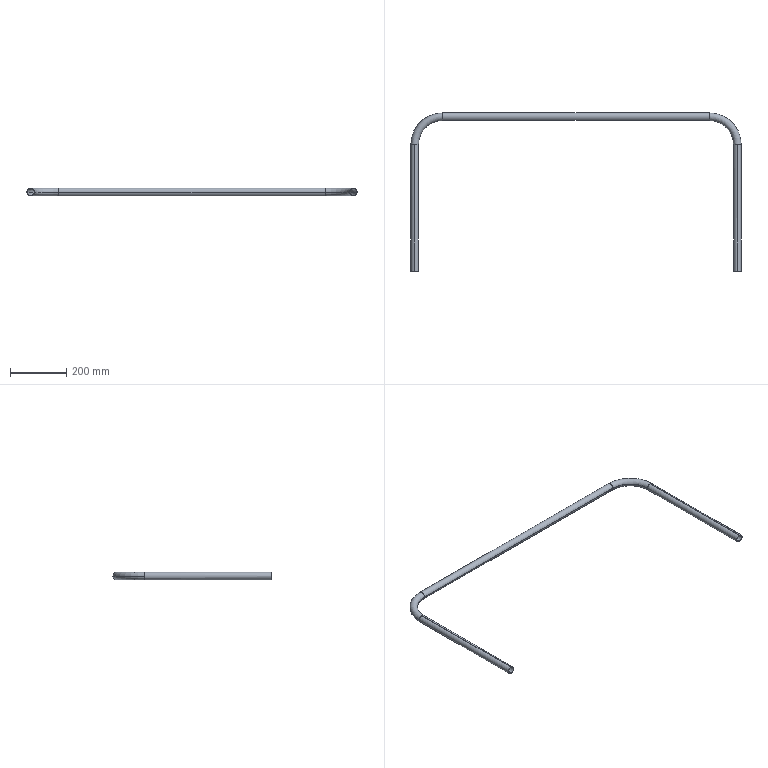Part | SolidWorks | features Sweep 1 | 1 solid | 22 faces | box 1177 x 563.5 x 27 mm | volume 176772 mm3 | cylinder 12 | torus 8 | plane 2 | commonest cylinder face diameters 25 x6 27 x6
STEP:
#1=CARTESIAN_POINT('',(-475.,562.5,0.));
#2=VERTEX_POINT('',#1);
#3=CARTESIAN_POINT('',(-475.,537.5,0.));
#4=VERTEX_POINT('',#3);
#5=CARTESIAN_POINT('',(-475.,550.,0.));
#6=DIRECTION('',(-1.,0.,0.));
#7=DIRECTION('',(0.,1.,0.));
#8=AXIS2_PLACEMENT_3D('',#5,#6,#7);
#9=CIRCLE('',#8,12.5);
#10=EDGE_CURVE('',#2,#4,#9,.T.);
#11=ORIENTED_EDGE('',*,*,#10,.F.);
#12=CARTESIAN_POINT('',(-587.5,450.,0.));
#13=VERTEX_POINT('',#12);
#14=CARTESIAN_POINT('',(-475.,450.,0.));
#15=DIRECTION('',(0.,0.,1.));
#16=DIRECTION('',(1.,0.,0.));
#17=AXIS2_PLACEMENT_3D('',#14,#15,#16);
#18=CIRCLE('',#17,112.5);
#19=EDGE_CURVE('',#2,#13,#18,.T.);
#20=ORIENTED_EDGE('',*,*,#19,.T.);
#21=CARTESIAN_POINT('',(-575.,450.,-12.5));
#22=VERTEX_POINT('',#21);
#23=CARTESIAN_POINT('',(-575.,450.,0.));
#24=DIRECTION('',(0.,-1.,0.));
#25=DIRECTION('',(0.,0.,-1.));
#26=AXIS2_PLACEMENT_3D('',#23,#24,#25);
#27=CIRCLE('',#26,12.5);
#28=EDGE_CURVE('',#13,#22,#27,.T.);
#29=ORIENTED_EDGE('',*,*,#28,.T.);
#30=CARTESIAN_POINT('',(-562.5,450.,0.));
#31=VERTEX_POINT('',#30);
#32=CARTESIAN_POINT('',(-575.,450.,0.));
#33=DIRECTION('',(0.,-1.,0.));
#34=DIRECTION('',(0.,0.,-1.));
#35=AXIS2_PLACEMENT_3D('',#32,#33,#34);
#36=CIRCLE('',#35,12.5);
#37=EDGE_CURVE('',#22,#31,#36,.T.);
#38=ORIENTED_EDGE('',*,*,#37,.T.);
#39=CARTESIAN_POINT('',(-475.,450.,0.));
#40=DIRECTION('',(0.,0.,1.));
#41=DIRECTION('',(1.,0.,0.));
#42=AXIS2_PLACEMENT_3D('',#39,#40,#41);
#43=CIRCLE('',#42,87.5);
#44=EDGE_CURVE('',#4,#31,#43,.T.);
#45=ORIENTED_EDGE('',*,*,#44,.F.);
#46=EDGE_LOOP('',(#11,#20,#29,#38,#45));
#47=FACE_OUTER_BOUND('',#46,.T.);
#48=CARTESIAN_POINT('',(-475.,450.,0.));
#49=DIRECTION('',(0.,0.,1.));
#50=DIRECTION('',(1.,0.,0.));
#51=AXIS2_PLACEMENT_3D('',#48,#49,#50);
#52=TOROIDAL_SURFACE('',#51,100.,12.5);
#53=ADVANCED_FACE('',(#47),#52,.F.);
#54=CARTESIAN_POINT('',(587.5,450.,0.));
#55=VERTEX_POINT('',#54);
#56=CARTESIAN_POINT('',(575.,450.,-12.5));
#57=VERTEX_POINT('',#56);
#58=CARTESIAN_POINT('',(575.,450.,0.));
#59=DIRECTION('',(0.,1.,0.));
#60=DIRECTION('',(1.,0.,0.));
#61=AXIS2_PLACEMENT_3D('',#58,#59,#60);
#62=CIRCLE('',#61,12.5);
#63=EDGE_CURVE('',#55,#57,#62,.T.);
#64=ORIENTED_EDGE('',*,*,#63,.F.);
#65=CARTESIAN_POINT('',(475.,562.5,0.));
#66=VERTEX_POINT('',#65);
#67=CARTESIAN_POINT('',(475.,450.,0.));
#68=DIRECTION('',(0.,0.,1.));
#69=DIRECTION('',(1.,0.,0.));
#70=AXIS2_PLACEMENT_3D('',#67,#68,#69);
#71=CIRCLE('',#70,112.5);
#72=EDGE_CURVE('',#55,#66,#71,.T.);
#73=ORIENTED_EDGE('',*,*,#72,.T.);
#74=CARTESIAN_POINT('',(475.,537.5,0.));
#75=VERTEX_POINT('',#74);
#76=CARTESIAN_POINT('',(475.,550.,0.));
#77=DIRECTION('',(-1.,0.,0.));
#78=DIRECTION('',(0.,-1.,0.));
#79=AXIS2_PLACEMENT_3D('',#76,#77,#78);
#80=CIRCLE('',#79,12.5);
#81=EDGE_CURVE('',#66,#75,#80,.T.);
#82=ORIENTED_EDGE('',*,*,#81,.T.);
#83=CARTESIAN_POINT('',(562.5,450.,0.));
#84=VERTEX_POINT('',#83);
#85=CARTESIAN_POINT('',(475.,450.,0.));
#86=DIRECTION('',(0.,0.,1.));
#87=DIRECTION('',(1.,0.,0.));
#88=AXIS2_PLACEMENT_3D('',#85,#86,#87);
#89=CIRCLE('',#88,87.5);
#90=EDGE_CURVE('',#84,#75,#89,.T.);
#91=ORIENTED_EDGE('',*,*,#90,.F.);
#92=CARTESIAN_POINT('',(575.,450.,0.));
#93=DIRECTION('',(0.,1.,0.));
#94=DIRECTION('',(1.,0.,0.));
#95=AXIS2_PLACEMENT_3D('',#92,#93,#94);
#96=CIRCLE('',#95,12.5);
#97=EDGE_CURVE('',#57,#84,#96,.T.);
#98=ORIENTED_EDGE('',*,*,#97,.F.);
#99=EDGE_LOOP('',(#64,#73,#82,#91,#98));
#100=FACE_OUTER_BOUND('',#99,.T.);
#101=CARTESIAN_POINT('',(475.,450.,0.));
#102=DIRECTION('',(0.,0.,1.));
#103=DIRECTION('',(1.,0.,0.));
#104=AXIS2_PLACEMENT_3D('',#101,#102,#103);
#105=TOROIDAL_SURFACE('',#104,100.,12.5);
#106=ADVANCED_FACE('',(#100),#105,.F.);
#107=CARTESIAN_POINT('',(-475.,536.5,0.));
#108=VERTEX_POINT('',#107);
#109=CARTESIAN_POINT('',(-475.,563.5,0.));
#110=VERTEX_POINT('',#109);
#111=CARTESIAN_POINT('',(-475.,550.,0.));
#112=DIRECTION('',(-1.,0.,0.));
#113=DIRECTION('',(0.,0.,1.));
#114=AXIS2_PLACEMENT_3D('',#111,#112,#113);
#115=CIRCLE('',#114,13.5);
#116=EDGE_CURVE('',#108,#110,#115,.T.);
#117=ORIENTED_EDGE('',*,*,#116,.T.);
#118=CARTESIAN_POINT('',(-588.5,450.,0.));
#119=VERTEX_POINT('',#118);
#120=CARTESIAN_POINT('',(-475.,450.,0.));
#121=DIRECTION('',(0.,0.,1.));
#122=DIRECTION('',(1.,0.,0.));
#123=AXIS2_PLACEMENT_3D('',#120,#121,#122);
#124=CIRCLE('',#123,113.5);
#125=EDGE_CURVE('',#110,#119,#124,.T.);
#126=ORIENTED_EDGE('',*,*,#125,.T.);
#127=CARTESIAN_POINT('',(-575.,450.,13.5));
#128=VERTEX_POINT('',#127);
#129=CARTESIAN_POINT('',(-575.,450.,0.));
#130=DIRECTION('',(0.,-1.,0.));
#131=DIRECTION('',(0.,0.,1.));
#132=AXIS2_PLACEMENT_3D('',#129,#130,#131);
#133=CIRCLE('',#132,13.5);
#134=EDGE_CURVE('',#128,#119,#133,.T.);
#135=ORIENTED_EDGE('',*,*,#134,.F.);
#136=CARTESIAN_POINT('',(-561.5,450.,0.));
#137=VERTEX_POINT('',#136);
#138=CARTESIAN_POINT('',(-575.,450.,0.));
#139=DIRECTION('',(0.,-1.,0.));
#140=DIRECTION('',(0.,0.,1.));
#141=AXIS2_PLACEMENT_3D('',#138,#139,#140);
#142=CIRCLE('',#141,13.5);
#143=EDGE_CURVE('',#137,#128,#142,.T.);
#144=ORIENTED_EDGE('',*,*,#143,.F.);
#145=CARTESIAN_POINT('',(-475.,450.,0.));
#146=DIRECTION('',(0.,0.,1.));
#147=DIRECTION('',(1.,0.,0.));
#148=AXIS2_PLACEMENT_3D('',#145,#146,#147);
#149=CIRCLE('',#148,86.5);
#150=EDGE_CURVE('',#108,#137,#149,.T.);
#151=ORIENTED_EDGE('',*,*,#150,.F.);
#152=EDGE_LOOP('',(#117,#126,#135,#144,#151));
#153=FACE_OUTER_BOUND('',#152,.T.);
#154=CARTESIAN_POINT('',(-475.,450.,0.));
#155=DIRECTION('',(0.,0.,1.));
#156=DIRECTION('',(1.,0.,0.));
#157=AXIS2_PLACEMENT_3D('',#154,#155,#156);
#158=TOROIDAL_SURFACE('',#157,100.,13.5);
#159=ADVANCED_FACE('',(#153),#158,.T.);
#160=CARTESIAN_POINT('',(575.,450.,13.5));
#161=VERTEX_POINT('',#160);
#162=CARTESIAN_POINT('',(588.5,450.,0.));
#163=VERTEX_POINT('',#162);
#164=CARTESIAN_POINT('',(575.,450.,0.));
#165=DIRECTION('',(0.,1.,0.));
#166=DIRECTION('',(0.,0.,1.));
#167=AXIS2_PLACEMENT_3D('',#164,#165,#166);
#168=CIRCLE('',#167,13.5);
#169=EDGE_CURVE('',#161,#163,#168,.T.);
#170=ORIENTED_EDGE('',*,*,#169,.T.);
#171=CARTESIAN_POINT('',(475.,563.5,0.));
#172=VERTEX_POINT('',#171);
#173=CARTESIAN_POINT('',(475.,450.,0.));
#174=DIRECTION('',(0.,0.,1.));
#175=DIRECTION('',(1.,0.,0.));
#176=AXIS2_PLACEMENT_3D('',#173,#174,#175);
#177=CIRCLE('',#176,113.5);
#178=EDGE_CURVE('',#163,#172,#177,.T.);
#179=ORIENTED_EDGE('',*,*,#178,.T.);
#180=CARTESIAN_POINT('',(475.,536.5,0.));
#181=VERTEX_POINT('',#180);
#182=CARTESIAN_POINT('',(475.,550.,0.));
#183=DIRECTION('',(-1.,0.,0.));
#184=DIRECTION('',(0.,0.,1.));
#185=AXIS2_PLACEMENT_3D('',#182,#183,#184);
#186=CIRCLE('',#185,13.5);
#187=EDGE_CURVE('',#181,#172,#186,.T.);
#188=ORIENTED_EDGE('',*,*,#187,.F.);
#189=CARTESIAN_POINT('',(561.5,450.,0.));
#190=VERTEX_POINT('',#189);
#191=CARTESIAN_POINT('',(475.,450.,0.));
#192=DIRECTION('',(0.,0.,1.));
#193=DIRECTION('',(1.,0.,0.));
#194=AXIS2_PLACEMENT_3D('',#191,#192,#193);
#195=CIRCLE('',#194,86.5);
#196=EDGE_CURVE('',#190,#181,#195,.T.);
#197=ORIENTED_EDGE('',*,*,#196,.F.);
#198=CARTESIAN_POINT('',(575.,450.,0.));
#199=DIRECTION('',(0.,1.,0.));
#200=DIRECTION('',(0.,0.,1.));
#201=AXIS2_PLACEMENT_3D('',#198,#199,#200);
#202=CIRCLE('',#201,13.5);
#203=EDGE_CURVE('',#190,#161,#202,.T.);
#204=ORIENTED_EDGE('',*,*,#203,.T.);
#205=EDGE_LOOP('',(#170,#179,#188,#197,#204));
#206=FACE_OUTER_BOUND('',#205,.T.);
#207=CARTESIAN_POINT('',(475.,450.,0.));
#208=DIRECTION('',(0.,0.,1.));
#209=DIRECTION('',(1.,0.,0.));
#210=AXIS2_PLACEMENT_3D('',#207,#208,#209);
#211=TOROIDAL_SURFACE('',#210,100.,13.5);
#212=ADVANCED_FACE('',(#206),#211,.T.);
#213=CARTESIAN_POINT('',(-575.,450.,12.5));
#214=VERTEX_POINT('',#213);
#215=CARTESIAN_POINT('',(-575.,450.,0.));
#216=DIRECTION('',(0.,-1.,0.));
#217=DIRECTION('',(0.,0.,-1.));
#218=AXIS2_PLACEMENT_3D('',#215,#216,#217);
#219=CIRCLE('',#218,12.5);
#220=EDGE_CURVE('',#214,#13,#219,.T.);
#221=ORIENTED_EDGE('',*,*,#220,.F.);
#222=CARTESIAN_POINT('',(-575.,0.,12.5));
#223=VERTEX_POINT('',#222);
#224=CARTESIAN_POINT('',(-575.,450.,12.5));
#225=DIRECTION('',(0.,-1.,0.));
#226=VECTOR('',#225,1000.);
#227=LINE('',#224,#226);
#228=EDGE_CURVE('',#214,#223,#227,.T.);
#229=ORIENTED_EDGE('',*,*,#228,.T.);
#230=CARTESIAN_POINT('',(-575.,0.,-12.5));
#231=VERTEX_POINT('',#230);
#232=CARTESIAN_POINT('',(-575.,0.,0.));
#233=DIRECTION('',(0.,-1.,0.));
#234=DIRECTION('',(0.,0.,-1.));
#235=AXIS2_PLACEMENT_3D('',#232,#233,#234);
#236=CIRCLE('',#235,12.5);
#237=EDGE_CURVE('',#223,#231,#236,.T.);
#238=ORIENTED_EDGE('',*,*,#237,.T.);
#239=CARTESIAN_POINT('',(-575.,450.,-12.5));
#240=DIRECTION('',(0.,-1.,0.));
#241=VECTOR('',#240,1000.);
#242=LINE('',#239,#241);
#243=EDGE_CURVE('',#22,#231,#242,.T.);
#244=ORIENTED_EDGE('',*,*,#243,.F.);
#245=ORIENTED_EDGE('',*,*,#28,.F.);
#246=EDGE_LOOP('',(#221,#229,#238,#244,#245));
#247=FACE_OUTER_BOUND('',#246,.T.);
#248=CARTESIAN_POINT('',(-575.,450.,0.));
#249=DIRECTION('',(0.,-1.,0.));
#250=DIRECTION('',(0.,0.,-1.));
#251=AXIS2_PLACEMENT_3D('',#248,#249,#250);
#252=CYLINDRICAL_SURFACE('',#251,12.5);
#253=ADVANCED_FACE('',(#247),#252,.F.);
#254=ORIENTED_EDGE('',*,*,#81,.F.);
#255=CARTESIAN_POINT('',(475.,562.5,0.));
#256=DIRECTION('',(-1.,0.,0.));
#257=VECTOR('',#256,1000.);
#258=LINE('',#255,#257);
#259=EDGE_CURVE('',#66,#2,#258,.T.);
#260=ORIENTED_EDGE('',*,*,#259,.T.);
#261=ORIENTED_EDGE('',*,*,#10,.T.);
#262=CARTESIAN_POINT('',(475.,537.5,0.));
#263=DIRECTION('',(-1.,0.,0.));
#264=VECTOR('',#263,1000.);
#265=LINE('',#262,#264);
#266=EDGE_CURVE('',#75,#4,#265,.T.);
#267=ORIENTED_EDGE('',*,*,#266,.F.);
#268=EDGE_LOOP('',(#254,#260,#261,#267));
#269=FACE_OUTER_BOUND('',#268,.T.);
#270=CARTESIAN_POINT('',(475.,550.,0.));
#271=DIRECTION('',(-1.,0.,0.));
#272=DIRECTION('',(0.,-1.,0.));
#273=AXIS2_PLACEMENT_3D('',#270,#271,#272);
#274=CYLINDRICAL_SURFACE('',#273,12.5);
#275=ADVANCED_FACE('',(#269),#274,.F.);
#276=CARTESIAN_POINT('',(575.,0.,-12.5));
#277=VERTEX_POINT('',#276);
#278=CARTESIAN_POINT('',(575.,0.,12.5));
#279=VERTEX_POINT('',#278);
#280=CARTESIAN_POINT('',(575.,0.,0.));
#281=DIRECTION('',(0.,1.,0.));
#282=DIRECTION('',(0.,0.,1.));
#283=AXIS2_PLACEMENT_3D('',#280,#281,#282);
#284=CIRCLE('',#283,12.5);
#285=EDGE_CURVE('',#277,#279,#284,.T.);
#286=ORIENTED_EDGE('',*,*,#285,.F.);
#287=CARTESIAN_POINT('',(575.,0.,-12.5));
#288=DIRECTION('',(0.,1.,0.));
#289=VECTOR('',#288,1000.);
#290=LINE('',#287,#289);
#291=EDGE_CURVE('',#277,#57,#290,.T.);
#292=ORIENTED_EDGE('',*,*,#291,.T.);
#293=ORIENTED_EDGE('',*,*,#97,.T.);
#294=CARTESIAN_POINT('',(575.,450.,12.5));
#295=VERTEX_POINT('',#294);
#296=CARTESIAN_POINT('',(575.,450.,0.));
#297=DIRECTION('',(0.,1.,0.));
#298=DIRECTION('',(1.,0.,0.));
#299=AXIS2_PLACEMENT_3D('',#296,#297,#298);
#300=CIRCLE('',#299,12.5);
#301=EDGE_CURVE('',#84,#295,#300,.T.);
#302=ORIENTED_EDGE('',*,*,#301,.T.);
#303=CARTESIAN_POINT('',(575.,0.,12.5));
#304=DIRECTION('',(0.,1.,0.));
#305=VECTOR('',#304,1000.);
#306=LINE('',#303,#305);
#307=EDGE_CURVE('',#279,#295,#306,.T.);
#308=ORIENTED_EDGE('',*,*,#307,.F.);
#309=EDGE_LOOP('',(#286,#292,#293,#302,#308));
#310=FACE_OUTER_BOUND('',#309,.T.);
#311=CARTESIAN_POINT('',(575.,0.,0.));
#312=DIRECTION('',(0.,1.,0.));
#313=DIRECTION('',(0.,0.,1.));
#314=AXIS2_PLACEMENT_3D('',#311,#312,#313);
#315=CYLINDRICAL_SURFACE('',#314,12.5);
#316=ADVANCED_FACE('',(#310),#315,.F.);
#317=CARTESIAN_POINT('',(-575.,450.,-13.5));
#318=VERTEX_POINT('',#317);
#319=CARTESIAN_POINT('',(-575.,450.,0.));
#320=DIRECTION('',(0.,-1.,0.));
#321=DIRECTION('',(0.,0.,1.));
#322=AXIS2_PLACEMENT_3D('',#319,#320,#321);
#323=CIRCLE('',#322,13.5);
#324=EDGE_CURVE('',#318,#137,#323,.T.);
#325=ORIENTED_EDGE('',*,*,#324,.T.);
#326=ORIENTED_EDGE('',*,*,#143,.T.);
#327=CARTESIAN_POINT('',(-575.,0.,13.5));
#328=VERTEX_POINT('',#327);
#329=CARTESIAN_POINT('',(-575.,450.,13.5));
#330=DIRECTION('',(0.,-1.,0.));
#331=VECTOR('',#330,1000.);
#332=LINE('',#329,#331);
#333=EDGE_CURVE('',#128,#328,#332,.T.);
#334=ORIENTED_EDGE('',*,*,#333,.T.);
#335=CARTESIAN_POINT('',(-575.,0.,-13.5));
#336=VERTEX_POINT('',#335);
#337=CARTESIAN_POINT('',(-575.,0.,0.));
#338=DIRECTION('',(0.,-1.,0.));
#339=DIRECTION('',(0.,0.,1.));
#340=AXIS2_PLACEMENT_3D('',#337,#338,#339);
#341=CIRCLE('',#340,13.5);
#342=EDGE_CURVE('',#336,#328,#341,.T.);
#343=ORIENTED_EDGE('',*,*,#342,.F.);
#344=CARTESIAN_POINT('',(-575.,450.,-13.5));
#345=DIRECTION('',(0.,-1.,0.));
#346=VECTOR('',#345,1000.);
#347=LINE('',#344,#346);
#348=EDGE_CURVE('',#318,#336,#347,.T.);
#349=ORIENTED_EDGE('',*,*,#348,.F.);
#350=EDGE_LOOP('',(#325,#326,#334,#343,#349));
#351=FACE_OUTER_BOUND('',#350,.T.);
#352=CARTESIAN_POINT('',(-575.,450.,0.));
#353=DIRECTION('',(0.,-1.,0.));
#354=DIRECTION('',(0.,0.,-1.));
#355=AXIS2_PLACEMENT_3D('',#352,#353,#354);
#356=CYLINDRICAL_SURFACE('',#355,13.5);
#357=ADVANCED_FACE('',(#351),#356,.T.);
#358=ORIENTED_EDGE('',*,*,#187,.T.);
#359=CARTESIAN_POINT('',(475.,563.5,0.));
#360=DIRECTION('',(-1.,0.,0.));
#361=VECTOR('',#360,1000.);
#362=LINE('',#359,#361);
#363=EDGE_CURVE('',#172,#110,#362,.T.);
#364=ORIENTED_EDGE('',*,*,#363,.T.);
#365=ORIENTED_EDGE('',*,*,#116,.F.);
#366=CARTESIAN_POINT('',(475.,536.5,0.));
#367=DIRECTION('',(-1.,0.,0.));
#368=VECTOR('',#367,1000.);
#369=LINE('',#366,#368);
#370=EDGE_CURVE('',#181,#108,#369,.T.);
#371=ORIENTED_EDGE('',*,*,#370,.F.);
#372=EDGE_LOOP('',(#358,#364,#365,#371));
#373=FACE_OUTER_BOUND('',#372,.T.);
#374=CARTESIAN_POINT('',(475.,550.,0.));
#375=DIRECTION('',(-1.,0.,0.));
#376=DIRECTION('',(0.,-1.,0.));
#377=AXIS2_PLACEMENT_3D('',#374,#375,#376);
#378=CYLINDRICAL_SURFACE('',#377,13.5);
#379=ADVANCED_FACE('',(#373),#378,.T.);
#380=CARTESIAN_POINT('',(575.,0.,13.5));
#381=VERTEX_POINT('',#380);
#382=CARTESIAN_POINT('',(575.,0.,-13.5));
#383=VERTEX_POINT('',#382);
#384=CARTESIAN_POINT('',(575.,0.,0.));
#385=DIRECTION('',(0.,1.,0.));
#386=DIRECTION('',(0.,0.,1.));
#387=AXIS2_PLACEMENT_3D('',#384,#385,#386);
#388=CIRCLE('',#387,13.5);
#389=EDGE_CURVE('',#381,#383,#388,.T.);
#390=ORIENTED_EDGE('',*,*,#389,.T.);
#391=CARTESIAN_POINT('',(575.,450.,-13.5));
#392=VERTEX_POINT('',#391);
#393=CARTESIAN_POINT('',(575.,0.,-13.5));
#394=DIRECTION('',(0.,1.,0.));
#395=VECTOR('',#394,1000.);
#396=LINE('',#393,#395);
#397=EDGE_CURVE('',#383,#392,#396,.T.);
#398=ORIENTED_EDGE('',*,*,#397,.T.);
#399=CARTESIAN_POINT('',(575.,450.,0.));
#400=DIRECTION('',(0.,1.,0.));
#401=DIRECTION('',(0.,0.,1.));
#402=AXIS2_PLACEMENT_3D('',#399,#400,#401);
#403=CIRCLE('',#402,13.5);
#404=EDGE_CURVE('',#163,#392,#403,.T.);
#405=ORIENTED_EDGE('',*,*,#404,.F.);
#406=ORIENTED_EDGE('',*,*,#169,.F.);
#407=CARTESIAN_POINT('',(575.,0.,13.5));
#408=DIRECTION('',(0.,1.,0.));
#409=VECTOR('',#408,1000.);
#410=LINE('',#407,#409);
#411=EDGE_CURVE('',#381,#161,#410,.T.);
#412=ORIENTED_EDGE('',*,*,#411,.F.);
#413=EDGE_LOOP('',(#390,#398,#405,#406,#412));
#414=FACE_OUTER_BOUND('',#413,.T.);
#415=CARTESIAN_POINT('',(575.,0.,0.));
#416=DIRECTION('',(0.,1.,0.));
#417=DIRECTION('',(0.,0.,1.));
#418=AXIS2_PLACEMENT_3D('',#415,#416,#417);
#419=CYLINDRICAL_SURFACE('',#418,13.5);
#420=ADVANCED_FACE('',(#414),#419,.T.);
#421=ORIENTED_EDGE('',*,*,#333,.F.);
#422=ORIENTED_EDGE('',*,*,#134,.T.);
#423=CARTESIAN_POINT('',(-575.,450.,0.));
#424=DIRECTION('',(0.,-1.,0.));
#425=DIRECTION('',(0.,0.,1.));
#426=AXIS2_PLACEMENT_3D('',#423,#424,#425);
#427=CIRCLE('',#426,13.5);
#428=EDGE_CURVE('',#119,#318,#427,.T.);
#429=ORIENTED_EDGE('',*,*,#428,.T.);
#430=ORIENTED_EDGE('',*,*,#348,.T.);
#431=CARTESIAN_POINT('',(-575.,0.,0.));
#432=DIRECTION('',(0.,-1.,0.));
#433=DIRECTION('',(0.,0.,1.));
#434=AXIS2_PLACEMENT_3D('',#431,#432,#433);
#435=CIRCLE('',#434,13.5);
#436=EDGE_CURVE('',#328,#336,#435,.T.);
#437=ORIENTED_EDGE('',*,*,#436,.F.);
#438=EDGE_LOOP('',(#421,#422,#429,#430,#437));
#439=FACE_OUTER_BOUND('',#438,.T.);
#440=CARTESIAN_POINT('',(-575.,450.,0.));
#441=DIRECTION('',(0.,-1.,0.));
#442=DIRECTION('',(0.,0.,-1.));
#443=AXIS2_PLACEMENT_3D('',#440,#441,#442);
#444=CYLINDRICAL_SURFACE('',#443,13.5);
#445=ADVANCED_FACE('',(#439),#444,.T.);
#446=ORIENTED_EDGE('',*,*,#125,.F.);
#447=CARTESIAN_POINT('',(-475.,550.,0.));
#448=DIRECTION('',(-1.,0.,0.));
#449=DIRECTION('',(0.,0.,1.));
#450=AXIS2_PLACEMENT_3D('',#447,#448,#449);
#451=CIRCLE('',#450,13.5);
#452=EDGE_CURVE('',#110,#108,#451,.T.);
#453=ORIENTED_EDGE('',*,*,#452,.T.);
#454=ORIENTED_EDGE('',*,*,#150,.T.);
#455=ORIENTED_EDGE('',*,*,#324,.F.);
#456=ORIENTED_EDGE('',*,*,#428,.F.);
#457=EDGE_LOOP('',(#446,#453,#454,#455,#456));
#458=FACE_OUTER_BOUND('',#457,.T.);
#459=CARTESIAN_POINT('',(-475.,450.,0.));
#460=DIRECTION('',(0.,0.,1.));
#461=DIRECTION('',(1.,0.,0.));
#462=AXIS2_PLACEMENT_3D('',#459,#460,#461);
#463=TOROIDAL_SURFACE('',#462,100.,13.5);
#464=ADVANCED_FACE('',(#458),#463,.T.);
#465=ORIENTED_EDGE('',*,*,#363,.F.);
#466=CARTESIAN_POINT('',(475.,550.,0.));
#467=DIRECTION('',(-1.,0.,0.));
#468=DIRECTION('',(0.,0.,1.));
#469=AXIS2_PLACEMENT_3D('',#466,#467,#468);
#470=CIRCLE('',#469,13.5);
#471=EDGE_CURVE('',#172,#181,#470,.T.);
#472=ORIENTED_EDGE('',*,*,#471,.T.);
#473=ORIENTED_EDGE('',*,*,#370,.T.);
#474=ORIENTED_EDGE('',*,*,#452,.F.);
#475=EDGE_LOOP('',(#465,#472,#473,#474));
#476=FACE_OUTER_BOUND('',#475,.T.);
#477=CARTESIAN_POINT('',(475.,550.,0.));
#478=DIRECTION('',(-1.,0.,0.));
#479=DIRECTION('',(0.,-1.,0.));
#480=AXIS2_PLACEMENT_3D('',#477,#478,#479);
#481=CYLINDRICAL_SURFACE('',#480,13.5);
#482=ADVANCED_FACE('',(#476),#481,.T.);
#483=ORIENTED_EDGE('',*,*,#178,.F.);
#484=ORIENTED_EDGE('',*,*,#404,.T.);
#485=CARTESIAN_POINT('',(575.,450.,0.));
#486=DIRECTION('',(0.,1.,0.));
#487=DIRECTION('',(0.,0.,1.));
#488=AXIS2_PLACEMENT_3D('',#485,#486,#487);
#489=CIRCLE('',#488,13.5);
#490=EDGE_CURVE('',#392,#190,#489,.T.);
#491=ORIENTED_EDGE('',*,*,#490,.T.);
#492=ORIENTED_EDGE('',*,*,#196,.T.);
#493=ORIENTED_EDGE('',*,*,#471,.F.);
#494=EDGE_LOOP('',(#483,#484,#491,#492,#493));
#495=FACE_OUTER_BOUND('',#494,.T.);
#496=CARTESIAN_POINT('',(475.,450.,0.));
#497=DIRECTION('',(0.,0.,1.));
#498=DIRECTION('',(1.,0.,0.));
#499=AXIS2_PLACEMENT_3D('',#496,#497,#498);
#500=TOROIDAL_SURFACE('',#499,100.,13.5);
#501=ADVANCED_FACE('',(#495),#500,.T.);
#502=ORIENTED_EDGE('',*,*,#397,.F.);
#503=CARTESIAN_POINT('',(575.,0.,0.));
#504=DIRECTION('',(0.,1.,0.));
#505=DIRECTION('',(0.,0.,1.));
#506=AXIS2_PLACEMENT_3D('',#503,#504,#505);
#507=CIRCLE('',#506,13.5);
#508=EDGE_CURVE('',#383,#381,#507,.T.);
#509=ORIENTED_EDGE('',*,*,#508,.T.);
#510=ORIENTED_EDGE('',*,*,#411,.T.);
#511=ORIENTED_EDGE('',*,*,#203,.F.);
#512=ORIENTED_EDGE('',*,*,#490,.F.);
#513=EDGE_LOOP('',(#502,#509,#510,#511,#512));
#514=FACE_OUTER_BOUND('',#513,.T.);
#515=CARTESIAN_POINT('',(575.,0.,0.));
#516=DIRECTION('',(0.,1.,0.));
#517=DIRECTION('',(0.,0.,1.));
#518=AXIS2_PLACEMENT_3D('',#515,#516,#517);
#519=CYLINDRICAL_SURFACE('',#518,13.5);
#520=ADVANCED_FACE('',(#514),#519,.T.);
#521=CARTESIAN_POINT('',(-575.,0.,0.));
#522=DIRECTION('',(0.,-1.,0.));
#523=DIRECTION('',(0.,0.,-1.));
#524=AXIS2_PLACEMENT_3D('',#521,#522,#523);
#525=CIRCLE('',#524,12.5);
#526=EDGE_CURVE('',#231,#223,#525,.T.);
#527=ORIENTED_EDGE('',*,*,#526,.F.);
#528=ORIENTED_EDGE('',*,*,#237,.F.);
#529=EDGE_LOOP('',(#527,#528));
#530=FACE_BOUND('',#529,.T.);
#531=ORIENTED_EDGE('',*,*,#342,.T.);
#532=ORIENTED_EDGE('',*,*,#436,.T.);
#533=EDGE_LOOP('',(#531,#532));
#534=FACE_OUTER_BOUND('',#533,.T.);
#535=CARTESIAN_POINT('',(-575.,0.,0.));
#536=DIRECTION('',(0.,-1.,0.));
#537=DIRECTION('',(0.,0.,1.));
#538=AXIS2_PLACEMENT_3D('',#535,#536,#537);
#539=PLANE('',#538);
#540=ADVANCED_FACE('',(#530,#534),#539,.T.);
#541=CARTESIAN_POINT('',(575.,0.,0.));
#542=DIRECTION('',(0.,1.,0.));
#543=DIRECTION('',(0.,0.,1.));
#544=AXIS2_PLACEMENT_3D('',#541,#542,#543);
#545=CIRCLE('',#544,12.5);
#546=EDGE_CURVE('',#279,#277,#545,.T.);
#547=ORIENTED_EDGE('',*,*,#546,.T.);
#548=ORIENTED_EDGE('',*,*,#285,.T.);
#549=EDGE_LOOP('',(#547,#548));
#550=FACE_BOUND('',#549,.T.);
#551=ORIENTED_EDGE('',*,*,#389,.F.);
#552=ORIENTED_EDGE('',*,*,#508,.F.);
#553=EDGE_LOOP('',(#551,#552));
#554=FACE_OUTER_BOUND('',#553,.T.);
#555=CARTESIAN_POINT('',(575.,0.,0.));
#556=DIRECTION('',(0.,1.,0.));
#557=DIRECTION('',(0.,0.,1.));
#558=AXIS2_PLACEMENT_3D('',#555,#556,#557);
#559=PLANE('',#558);
#560=ADVANCED_FACE('',(#550,#554),#559,.F.);
#561=ORIENTED_EDGE('',*,*,#228,.F.);
#562=CARTESIAN_POINT('',(-575.,450.,0.));
#563=DIRECTION('',(0.,-1.,0.));
#564=DIRECTION('',(0.,0.,-1.));
#565=AXIS2_PLACEMENT_3D('',#562,#563,#564);
#566=CIRCLE('',#565,12.5);
#567=EDGE_CURVE('',#31,#214,#566,.T.);
#568=ORIENTED_EDGE('',*,*,#567,.F.);
#569=ORIENTED_EDGE('',*,*,#37,.F.);
#570=ORIENTED_EDGE('',*,*,#243,.T.);
#571=ORIENTED_EDGE('',*,*,#526,.T.);
#572=EDGE_LOOP('',(#561,#568,#569,#570,#571));
#573=FACE_OUTER_BOUND('',#572,.T.);
#574=CARTESIAN_POINT('',(-575.,450.,0.));
#575=DIRECTION('',(0.,-1.,0.));
#576=DIRECTION('',(0.,0.,-1.));
#577=AXIS2_PLACEMENT_3D('',#574,#575,#576);
#578=CYLINDRICAL_SURFACE('',#577,12.5);
#579=ADVANCED_FACE('',(#573),#578,.F.);
#580=ORIENTED_EDGE('',*,*,#19,.F.);
#581=CARTESIAN_POINT('',(-475.,550.,0.));
#582=DIRECTION('',(-1.,0.,0.));
#583=DIRECTION('',(0.,1.,0.));
#584=AXIS2_PLACEMENT_3D('',#581,#582,#583);
#585=CIRCLE('',#584,12.5);
#586=EDGE_CURVE('',#4,#2,#585,.T.);
#587=ORIENTED_EDGE('',*,*,#586,.F.);
#588=ORIENTED_EDGE('',*,*,#44,.T.);
#589=ORIENTED_EDGE('',*,*,#567,.T.);
#590=ORIENTED_EDGE('',*,*,#220,.T.);
#591=EDGE_LOOP('',(#580,#587,#588,#589,#590));
#592=FACE_OUTER_BOUND('',#591,.T.);
#593=CARTESIAN_POINT('',(-475.,450.,0.));
#594=DIRECTION('',(0.,0.,1.));
#595=DIRECTION('',(1.,0.,0.));
#596=AXIS2_PLACEMENT_3D('',#593,#594,#595);
#597=TOROIDAL_SURFACE('',#596,100.,12.5);
#598=ADVANCED_FACE('',(#592),#597,.F.);
#599=ORIENTED_EDGE('',*,*,#259,.F.);
#600=CARTESIAN_POINT('',(475.,550.,0.));
#601=DIRECTION('',(-1.,0.,0.));
#602=DIRECTION('',(0.,-1.,0.));
#603=AXIS2_PLACEMENT_3D('',#600,#601,#602);
#604=CIRCLE('',#603,12.5);
#605=EDGE_CURVE('',#75,#66,#604,.T.);
#606=ORIENTED_EDGE('',*,*,#605,.F.);
#607=ORIENTED_EDGE('',*,*,#266,.T.);
#608=ORIENTED_EDGE('',*,*,#586,.T.);
#609=EDGE_LOOP('',(#599,#606,#607,#608));
#610=FACE_OUTER_BOUND('',#609,.T.);
#611=CARTESIAN_POINT('',(475.,550.,0.));
#612=DIRECTION('',(-1.,0.,0.));
#613=DIRECTION('',(0.,-1.,0.));
#614=AXIS2_PLACEMENT_3D('',#611,#612,#613);
#615=CYLINDRICAL_SURFACE('',#614,12.5);
#616=ADVANCED_FACE('',(#610),#615,.F.);
#617=ORIENTED_EDGE('',*,*,#72,.F.);
#618=CARTESIAN_POINT('',(575.,450.,0.));
#619=DIRECTION('',(0.,1.,0.));
#620=DIRECTION('',(1.,0.,0.));
#621=AXIS2_PLACEMENT_3D('',#618,#619,#620);
#622=CIRCLE('',#621,12.5);
#623=EDGE_CURVE('',#295,#55,#622,.T.);
#624=ORIENTED_EDGE('',*,*,#623,.F.);
#625=ORIENTED_EDGE('',*,*,#301,.F.);
#626=ORIENTED_EDGE('',*,*,#90,.T.);
#627=ORIENTED_EDGE('',*,*,#605,.T.);
#628=EDGE_LOOP('',(#617,#624,#625,#626,#627));
#629=FACE_OUTER_BOUND('',#628,.T.);
#630=CARTESIAN_POINT('',(475.,450.,0.));
#631=DIRECTION('',(0.,0.,1.));
#632=DIRECTION('',(1.,0.,0.));
#633=AXIS2_PLACEMENT_3D('',#630,#631,#632);
#634=TOROIDAL_SURFACE('',#633,100.,12.5);
#635=ADVANCED_FACE('',(#629),#634,.F.);
#636=ORIENTED_EDGE('',*,*,#291,.F.);
#637=ORIENTED_EDGE('',*,*,#546,.F.);
#638=ORIENTED_EDGE('',*,*,#307,.T.);
#639=ORIENTED_EDGE('',*,*,#623,.T.);
#640=ORIENTED_EDGE('',*,*,#63,.T.);
#641=EDGE_LOOP('',(#636,#637,#638,#639,#640));
#642=FACE_OUTER_BOUND('',#641,.T.);
#643=CARTESIAN_POINT('',(575.,0.,0.));
#644=DIRECTION('',(0.,1.,0.));
#645=DIRECTION('',(0.,0.,1.));
#646=AXIS2_PLACEMENT_3D('',#643,#644,#645);
#647=CYLINDRICAL_SURFACE('',#646,12.5);
#648=ADVANCED_FACE('',(#642),#647,.F.);
#649=CLOSED_SHELL('',(#53,#106,#159,#212,#253,#275,#316,#357,#379,#420,#445,#464,#482,#501,#520,#540,#560,#579,#598,#616,#635,#648));
#650=MANIFOLD_SOLID_BREP('',#649);
#651=CARTESIAN_POINT('',(0.,0.,0.));
#652=DIRECTION('',(0.,0.,1.));
#653=DIRECTION('',(1.,0.,0.));
#654=AXIS2_PLACEMENT_3D('',#651,#652,#653);
#655=(LENGTH_UNIT()NAMED_UNIT(*)SI_UNIT(.MILLI.,.METRE.));
#656=UNCERTAINTY_MEASURE_WITH_UNIT(LENGTH_MEASURE(0.00001),#655,'','');
#657=(NAMED_UNIT(*)PLANE_ANGLE_UNIT()SI_UNIT($,.RADIAN.));
#658=(NAMED_UNIT(*)SI_UNIT($,.STERADIAN.)SOLID_ANGLE_UNIT());
#659=(GEOMETRIC_REPRESENTATION_CONTEXT(3)GLOBAL_UNCERTAINTY_ASSIGNED_CONTEXT((#656))GLOBAL_UNIT_ASSIGNED_CONTEXT((#655,#657,#658))REPRESENTATION_CONTEXT('',''));
#660=ADVANCED_BREP_SHAPE_REPRESENTATION('',(#650,#654),#659);